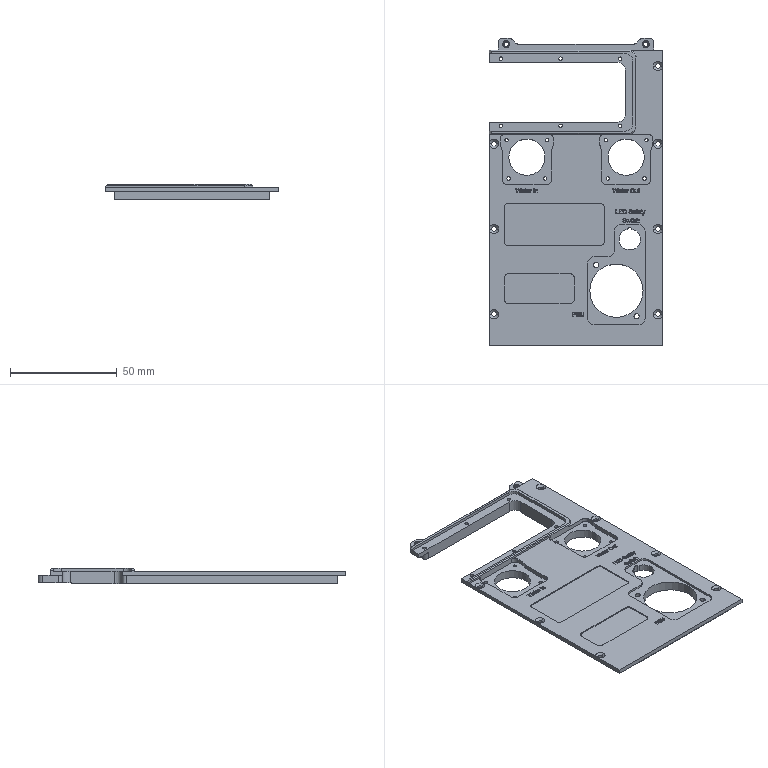NC program | NX | posted with a generic post | part box 81.5 x 144.28 x 7.5 mm
Lines 1 to 90 of 9048:
N10 G17 G21 G94 G90
(FLOOR_FACING , TOOL : D63面刀)
N12 T11 M6
N14 G54
N16 G17 G0 G90 X113.64 Y-25. S4500 M3
N18 G43 Z50. H11
N20 Z3.
N22 G94 G1 Z0. F800.
N24 X103.64
N26 X-103.64
N28 Y15.55
N30 X103.64
N32 X113.64
N34 Z3.
N36 G0 Z50.
N38 M5
(DRILLING , TOOL : 倒角-3.)
N40 T03 M6
N42 G54
N44 G17 G0 G90 X62.602 Y20.75 S3000 M3
N46 G43 Z10. H3
N48 G94 G81 G98 Z-1.5 F150. R2.5
N50 Y-7.25
N52 Y-35.25
N54 X31.102 Z-1. R3.
N56 X24.34 Y-32.55
N58 X6.34 Y-31.65
N60 Y-14.45
N62 X16.34 Y-23.05
N64 X24.34 Y-13.55
N66 X31.102 Y-7.25
N68 X24.34 Y14.05
N70 X31.102 Y20.75
N72 X24.34 Y33.05
N74 X16.34 Y23.55
N76 X6.34 Y32.15
N78 Y14.95
N80 G80
N82 G0 X6.34 Y14.95 Z10.
(DRILLING_COPY_1 , TOOL : 倒角-3.)
N84 X69.36 Y32.75
N86 G81 Z-1.8 F150. R2.5
N88 Y-32.75
N90 G80
N92 G0 X69.36 Y-32.75 Z10.
N94 M5
(DRILLING_COPY_1_COPY , TOOL : Z2.3)
N96 T06 M6
N98 G54
N100 G17 G0 G90 X69.36 Y32.75 S3000 M3
N102 G43 Z10. H6
N104 G94 G83 G98 Z-10.5 F200. Q2. R2.5
N106 Y-32.75
N108 G80
N110 G0 X69.36 Y-32.75 Z10.
N112 M5
(DRILLING_COPY , TOOL : Z1.85)
N114 T04 M6
N116 G54
N118 G17 G0 G90 X62.602 Y20.75 S3000 M3
N120 G43 Z10. H4
N122 G94 G83 G98 Z-9.5 F200. Q2. R2.5
N124 Y-7.25
N126 Y-35.25
N128 X31.102 Z-9. R3.
N130 X24.34 Y-32.55
N132 X6.34 Y-31.65
N134 Y-14.45
N136 X24.34 Y-13.55
N138 X31.102 Y-7.25
N140 X24.34 Y14.05
N142 X31.102 Y20.75
N144 X24.34 Y33.05
N146 X6.34 Y32.15
N148 Y14.95
N150 G80
N152 G0 X6.34 Y14.95 Z10.
N154 M5